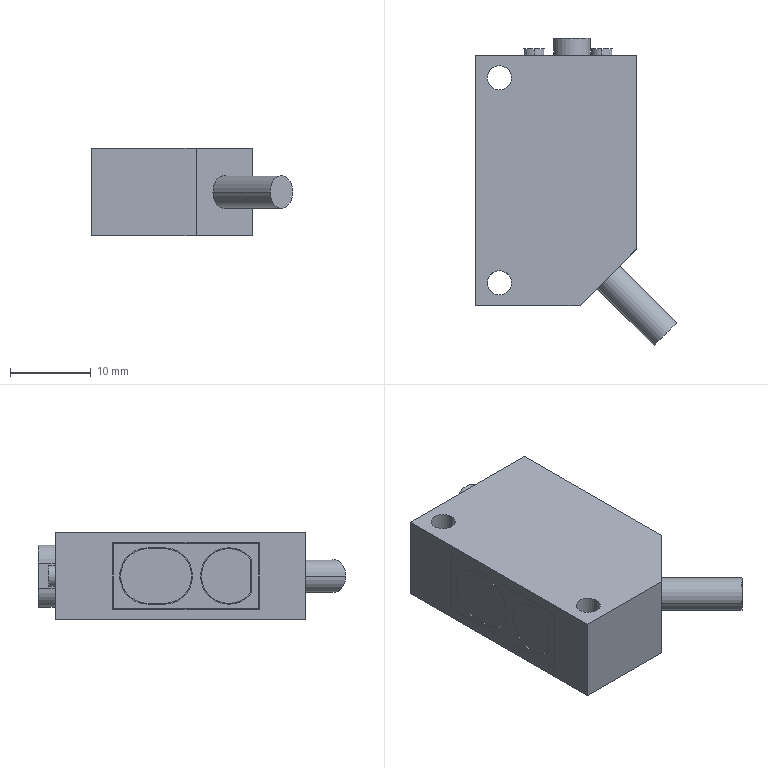Part | STEP file | Photoelectric SensorE3Z_LS61 | 1 solid | 68 faces | box 24.985 x 38.085 x 10.8 mm | volume 6465 mm3 | plane 37 | cylinder 31 | commonest cylinder face diameters 6.8 x5 7 x5 2.6 x4 2.9 x4 3 x4 3.1 x4